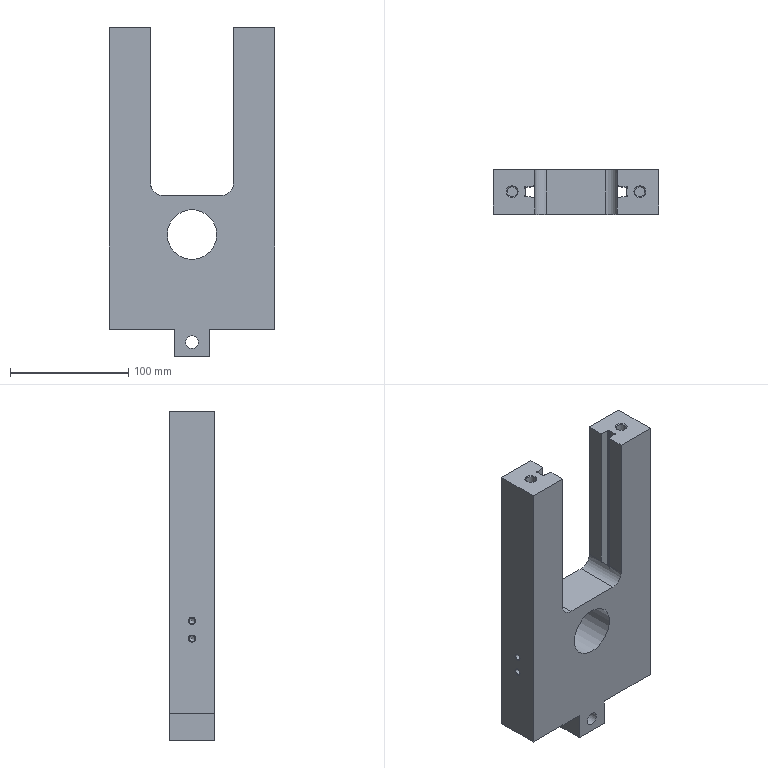Part | STEP file | 冲床-300配套压波_id962_x_t | 1 solid | 69 faces | box 140 x 38 x 278 mm | volume 905448 mm3 | plane 29 | cylinder 26 | cone 14 | commonest cylinder face diameters 4 x8 1 x4 8.5 x4 4.2 x3 5 x2 20 x2